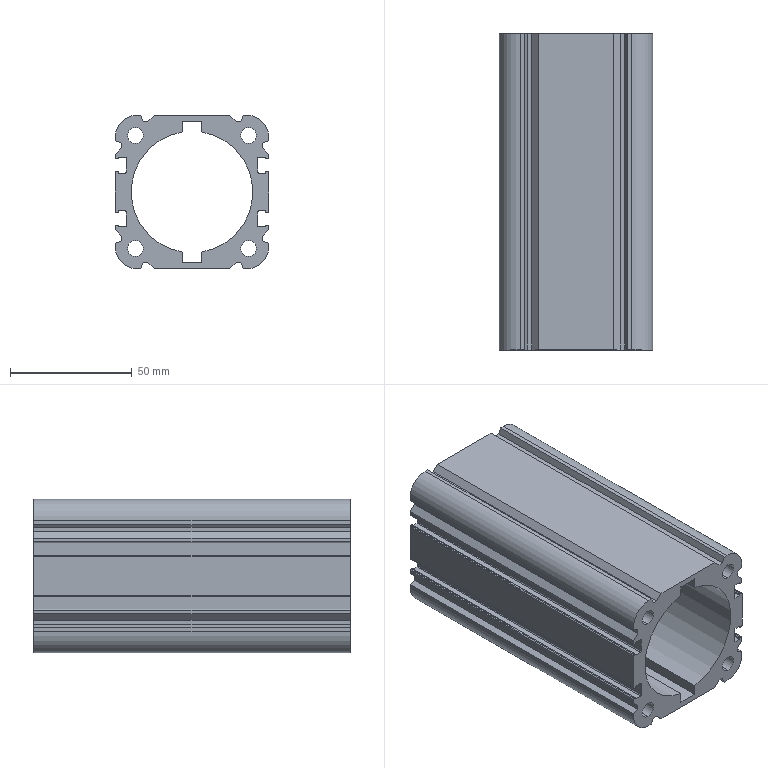Part | STEP file | 1 solid | 122 faces | box 63 x 130 x 63 mm | volume 202293 mm3 | plane 76 | cylinder 46 | commonest cylinder face diameters 0.6 x16 0.8 x16 6.5 x8 17.5 x4 50 x2